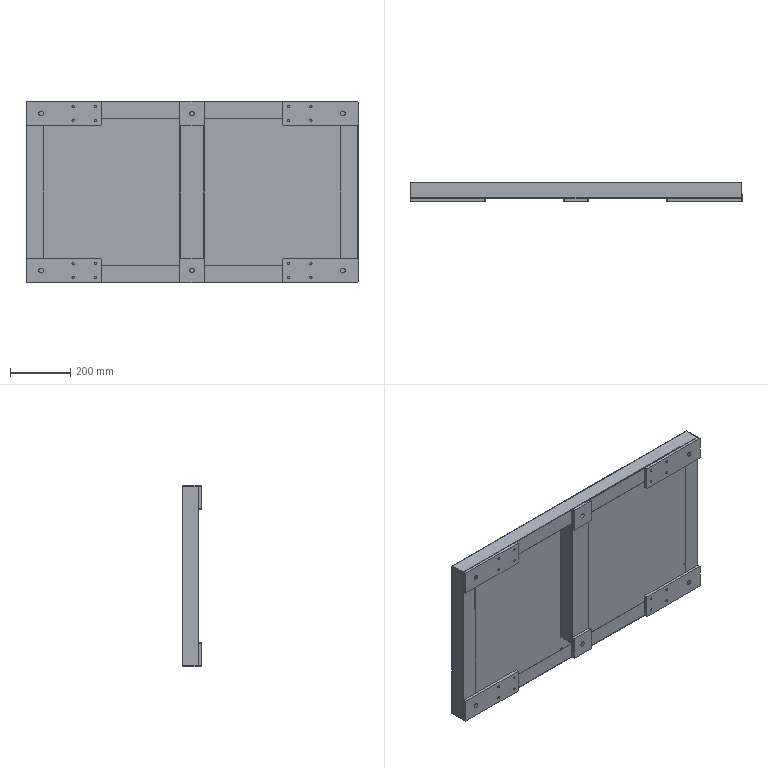Part | SolidWorks | 10 solids | 303 faces | box 1100 x 63 x 600.001 mm | volume 2743089 mm3 | plane 167 | cylinder 120 | spline 16 | commonest cylinder face diameters 7.5 x32 4.5 x20 10 x16 15.5 x14 20 x14 0.2 x12